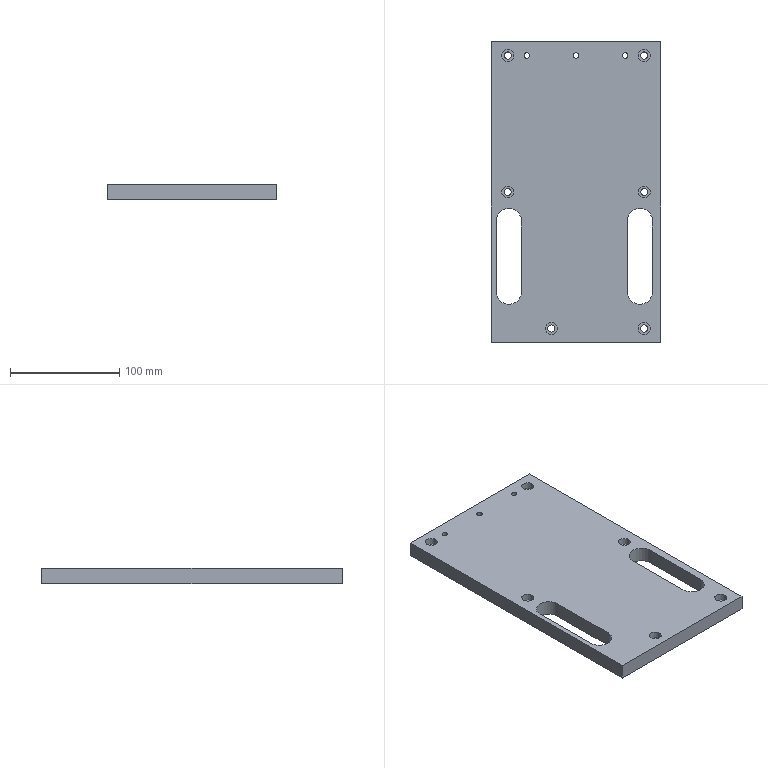Part | STEP file | 0232_212_Work_Base | 1 solid | 50 faces | box 155 x 275 x 14 mm | volume 537232 mm3 | cylinder 34 | plane 16 | commonest cylinder face diameters 6.5 x12 11 x12 5 x6 23 x4